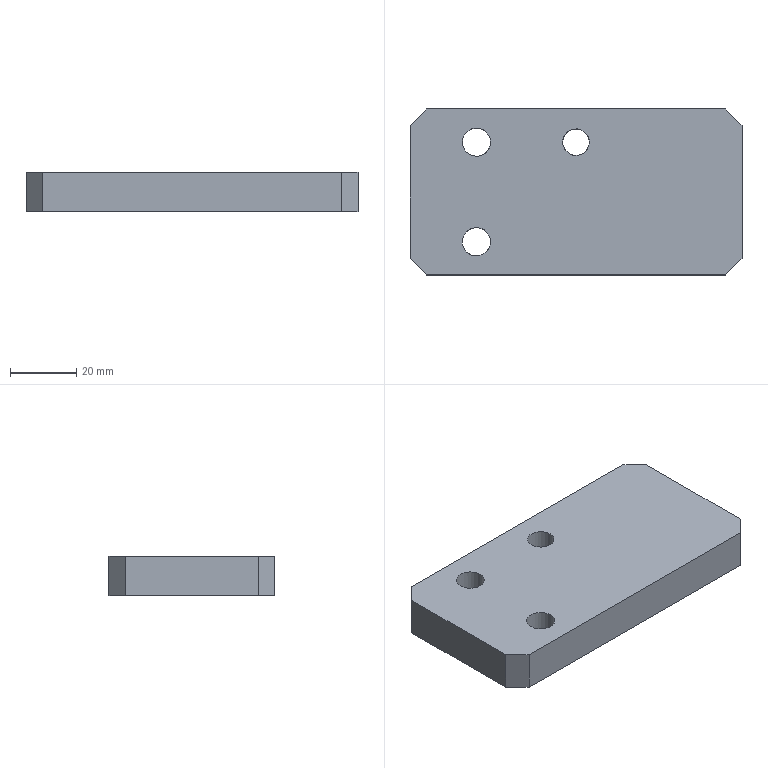Part | NX | features BREP 1 | 1 solid | 13 faces | box 100 x 50 x 12 mm | volume 57435 mm3 | plane 10 | cylinder 3 | commonest cylinder face diameters 8.5 x2 8 x1
STEP:
#1=CARTESIAN_POINT('',(50.,-20.,12.));
#2=VERTEX_POINT('',#1);
#3=CARTESIAN_POINT('',(50.,20.,12.));
#4=VERTEX_POINT('',#3);
#5=CARTESIAN_POINT('',(50.,25.,12.));
#6=DIRECTION('',(0.,1.,0.));
#7=VECTOR('',#6,1000.);
#8=LINE('',#5,#7);
#9=EDGE_CURVE('',#2,#4,#8,.T.);
#10=ORIENTED_EDGE('',*,*,#9,.F.);
#11=CARTESIAN_POINT('',(50.,-20.,0.));
#12=VERTEX_POINT('',#11);
#13=CARTESIAN_POINT('',(50.,-20.,15.));
#14=DIRECTION('',(0.,0.,-1.));
#15=VECTOR('',#14,1000.);
#16=LINE('',#13,#15);
#17=EDGE_CURVE('',#2,#12,#16,.T.);
#18=ORIENTED_EDGE('',*,*,#17,.T.);
#19=CARTESIAN_POINT('',(50.,20.,0.));
#20=VERTEX_POINT('',#19);
#21=CARTESIAN_POINT('',(50.,25.,0.));
#22=DIRECTION('',(0.,1.,0.));
#23=VECTOR('',#22,1000.);
#24=LINE('',#21,#23);
#25=EDGE_CURVE('',#12,#20,#24,.T.);
#26=ORIENTED_EDGE('',*,*,#25,.T.);
#27=CARTESIAN_POINT('',(50.,20.,15.));
#28=DIRECTION('',(0.,0.,1.));
#29=VECTOR('',#28,1000.);
#30=LINE('',#27,#29);
#31=EDGE_CURVE('',#20,#4,#30,.T.);
#32=ORIENTED_EDGE('',*,*,#31,.T.);
#33=EDGE_LOOP('',(#10,#18,#26,#32));
#34=FACE_BOUND('',#33,.T.);
#35=CARTESIAN_POINT('',(50.,25.,15.));
#36=DIRECTION('',(-1.,0.,0.));
#37=DIRECTION('',(0.,0.,-1.));
#38=AXIS2_PLACEMENT_3D('',#35,#36,#37);
#39=PLANE('',#38);
#40=ADVANCED_FACE('',(#34),#39,.F.);
#41=CARTESIAN_POINT('',(45.,25.,12.));
#42=VERTEX_POINT('',#41);
#43=CARTESIAN_POINT('',(-45.,25.,12.));
#44=VERTEX_POINT('',#43);
#45=CARTESIAN_POINT('',(-50.,25.,12.));
#46=DIRECTION('',(-1.,0.,0.));
#47=VECTOR('',#46,1000.);
#48=LINE('',#45,#47);
#49=EDGE_CURVE('',#42,#44,#48,.T.);
#50=ORIENTED_EDGE('',*,*,#49,.F.);
#51=CARTESIAN_POINT('',(45.,25.,0.));
#52=VERTEX_POINT('',#51);
#53=CARTESIAN_POINT('',(45.,25.,15.));
#54=DIRECTION('',(0.,0.,-1.));
#55=VECTOR('',#54,1000.);
#56=LINE('',#53,#55);
#57=EDGE_CURVE('',#42,#52,#56,.T.);
#58=ORIENTED_EDGE('',*,*,#57,.T.);
#59=CARTESIAN_POINT('',(-45.,25.,0.));
#60=VERTEX_POINT('',#59);
#61=CARTESIAN_POINT('',(-50.,25.,0.));
#62=DIRECTION('',(-1.,0.,0.));
#63=VECTOR('',#62,1000.);
#64=LINE('',#61,#63);
#65=EDGE_CURVE('',#52,#60,#64,.T.);
#66=ORIENTED_EDGE('',*,*,#65,.T.);
#67=CARTESIAN_POINT('',(-45.,25.,15.));
#68=DIRECTION('',(0.,0.,1.));
#69=VECTOR('',#68,1000.);
#70=LINE('',#67,#69);
#71=EDGE_CURVE('',#60,#44,#70,.T.);
#72=ORIENTED_EDGE('',*,*,#71,.T.);
#73=EDGE_LOOP('',(#50,#58,#66,#72));
#74=FACE_BOUND('',#73,.T.);
#75=CARTESIAN_POINT('',(-50.,25.,15.));
#76=DIRECTION('',(0.,-1.,0.));
#77=DIRECTION('',(0.,0.,1.));
#78=AXIS2_PLACEMENT_3D('',#75,#76,#77);
#79=PLANE('',#78);
#80=ADVANCED_FACE('',(#74),#79,.F.);
#81=CARTESIAN_POINT('',(-50.,20.,12.));
#82=VERTEX_POINT('',#81);
#83=CARTESIAN_POINT('',(-50.,-20.,12.));
#84=VERTEX_POINT('',#83);
#85=CARTESIAN_POINT('',(-50.,25.,12.));
#86=DIRECTION('',(0.,-1.,0.));
#87=VECTOR('',#86,1000.);
#88=LINE('',#85,#87);
#89=EDGE_CURVE('',#82,#84,#88,.T.);
#90=ORIENTED_EDGE('',*,*,#89,.F.);
#91=CARTESIAN_POINT('',(-50.,20.,0.));
#92=VERTEX_POINT('',#91);
#93=CARTESIAN_POINT('',(-50.,20.,15.));
#94=DIRECTION('',(0.,0.,-1.));
#95=VECTOR('',#94,1000.);
#96=LINE('',#93,#95);
#97=EDGE_CURVE('',#82,#92,#96,.T.);
#98=ORIENTED_EDGE('',*,*,#97,.T.);
#99=CARTESIAN_POINT('',(-50.,-20.,0.));
#100=VERTEX_POINT('',#99);
#101=CARTESIAN_POINT('',(-50.,25.,0.));
#102=DIRECTION('',(0.,-1.,0.));
#103=VECTOR('',#102,1000.);
#104=LINE('',#101,#103);
#105=EDGE_CURVE('',#92,#100,#104,.T.);
#106=ORIENTED_EDGE('',*,*,#105,.T.);
#107=CARTESIAN_POINT('',(-50.,-20.,15.));
#108=DIRECTION('',(0.,0.,1.));
#109=VECTOR('',#108,1000.);
#110=LINE('',#107,#109);
#111=EDGE_CURVE('',#100,#84,#110,.T.);
#112=ORIENTED_EDGE('',*,*,#111,.T.);
#113=EDGE_LOOP('',(#90,#98,#106,#112));
#114=FACE_BOUND('',#113,.T.);
#115=CARTESIAN_POINT('',(-50.,25.,15.));
#116=DIRECTION('',(1.,0.,0.));
#117=DIRECTION('',(0.,0.,1.));
#118=AXIS2_PLACEMENT_3D('',#115,#116,#117);
#119=PLANE('',#118);
#120=ADVANCED_FACE('',(#114),#119,.F.);
#121=CARTESIAN_POINT('',(-45.,-25.,12.));
#122=VERTEX_POINT('',#121);
#123=CARTESIAN_POINT('',(45.,-25.,12.));
#124=VERTEX_POINT('',#123);
#125=CARTESIAN_POINT('',(-50.,-25.,12.));
#126=DIRECTION('',(1.,0.,0.));
#127=VECTOR('',#126,1000.);
#128=LINE('',#125,#127);
#129=EDGE_CURVE('',#122,#124,#128,.T.);
#130=ORIENTED_EDGE('',*,*,#129,.F.);
#131=CARTESIAN_POINT('',(-45.,-25.,0.));
#132=VERTEX_POINT('',#131);
#133=CARTESIAN_POINT('',(-45.,-25.,15.));
#134=DIRECTION('',(0.,0.,-1.));
#135=VECTOR('',#134,1000.);
#136=LINE('',#133,#135);
#137=EDGE_CURVE('',#122,#132,#136,.T.);
#138=ORIENTED_EDGE('',*,*,#137,.T.);
#139=CARTESIAN_POINT('',(45.,-25.,0.));
#140=VERTEX_POINT('',#139);
#141=CARTESIAN_POINT('',(-50.,-25.,0.));
#142=DIRECTION('',(1.,0.,0.));
#143=VECTOR('',#142,1000.);
#144=LINE('',#141,#143);
#145=EDGE_CURVE('',#132,#140,#144,.T.);
#146=ORIENTED_EDGE('',*,*,#145,.T.);
#147=CARTESIAN_POINT('',(45.,-25.,15.));
#148=DIRECTION('',(0.,0.,1.));
#149=VECTOR('',#148,1000.);
#150=LINE('',#147,#149);
#151=EDGE_CURVE('',#140,#124,#150,.T.);
#152=ORIENTED_EDGE('',*,*,#151,.T.);
#153=EDGE_LOOP('',(#130,#138,#146,#152));
#154=FACE_BOUND('',#153,.T.);
#155=CARTESIAN_POINT('',(-50.,-25.,15.));
#156=DIRECTION('',(0.,1.,0.));
#157=DIRECTION('',(0.,0.,-1.));
#158=AXIS2_PLACEMENT_3D('',#155,#156,#157);
#159=PLANE('',#158);
#160=ADVANCED_FACE('',(#154),#159,.F.);
#161=ORIENTED_EDGE('',*,*,#137,.F.);
#162=CARTESIAN_POINT('',(-45.,-25.,12.));
#163=DIRECTION('',(-0.7071,0.7071,0.));
#164=VECTOR('',#163,1000.);
#165=LINE('',#162,#164);
#166=EDGE_CURVE('',#122,#84,#165,.T.);
#167=ORIENTED_EDGE('',*,*,#166,.T.);
#168=ORIENTED_EDGE('',*,*,#111,.F.);
#169=CARTESIAN_POINT('',(-45.,-25.,0.));
#170=DIRECTION('',(-0.7071,0.7071,0.));
#171=VECTOR('',#170,1000.);
#172=LINE('',#169,#171);
#173=EDGE_CURVE('',#132,#100,#172,.T.);
#174=ORIENTED_EDGE('',*,*,#173,.F.);
#175=EDGE_LOOP('',(#161,#167,#168,#174));
#176=FACE_BOUND('',#175,.T.);
#177=CARTESIAN_POINT('',(-45.,-25.,15.));
#178=DIRECTION('',(0.7071,0.7071,0.));
#179=DIRECTION('',(0.,0.,1.));
#180=AXIS2_PLACEMENT_3D('',#177,#178,#179);
#181=PLANE('',#180);
#182=ADVANCED_FACE('',(#176),#181,.F.);
#183=ORIENTED_EDGE('',*,*,#97,.F.);
#184=CARTESIAN_POINT('',(-50.,20.,12.));
#185=DIRECTION('',(0.7071,0.7071,0.));
#186=VECTOR('',#185,1000.);
#187=LINE('',#184,#186);
#188=EDGE_CURVE('',#82,#44,#187,.T.);
#189=ORIENTED_EDGE('',*,*,#188,.T.);
#190=ORIENTED_EDGE('',*,*,#71,.F.);
#191=CARTESIAN_POINT('',(-50.,20.,0.));
#192=DIRECTION('',(0.7071,0.7071,0.));
#193=VECTOR('',#192,1000.);
#194=LINE('',#191,#193);
#195=EDGE_CURVE('',#92,#60,#194,.T.);
#196=ORIENTED_EDGE('',*,*,#195,.F.);
#197=EDGE_LOOP('',(#183,#189,#190,#196));
#198=FACE_BOUND('',#197,.T.);
#199=CARTESIAN_POINT('',(-50.,20.,15.));
#200=DIRECTION('',(0.7071,-0.7071,0.));
#201=DIRECTION('',(0.,0.,1.));
#202=AXIS2_PLACEMENT_3D('',#199,#200,#201);
#203=PLANE('',#202);
#204=ADVANCED_FACE('',(#198),#203,.F.);
#205=ORIENTED_EDGE('',*,*,#17,.F.);
#206=CARTESIAN_POINT('',(50.,-20.,12.));
#207=DIRECTION('',(-0.7071,-0.7071,0.));
#208=VECTOR('',#207,1000.);
#209=LINE('',#206,#208);
#210=EDGE_CURVE('',#2,#124,#209,.T.);
#211=ORIENTED_EDGE('',*,*,#210,.T.);
#212=ORIENTED_EDGE('',*,*,#151,.F.);
#213=CARTESIAN_POINT('',(50.,-20.,0.));
#214=DIRECTION('',(-0.7071,-0.7071,0.));
#215=VECTOR('',#214,1000.);
#216=LINE('',#213,#215);
#217=EDGE_CURVE('',#12,#140,#216,.T.);
#218=ORIENTED_EDGE('',*,*,#217,.F.);
#219=EDGE_LOOP('',(#205,#211,#212,#218));
#220=FACE_BOUND('',#219,.T.);
#221=CARTESIAN_POINT('',(50.,-20.,15.));
#222=DIRECTION('',(-0.7071,0.7071,0.));
#223=DIRECTION('',(0.,0.,1.));
#224=AXIS2_PLACEMENT_3D('',#221,#222,#223);
#225=PLANE('',#224);
#226=ADVANCED_FACE('',(#220),#225,.F.);
#227=ORIENTED_EDGE('',*,*,#57,.F.);
#228=CARTESIAN_POINT('',(45.,25.,12.));
#229=DIRECTION('',(0.7071,-0.7071,0.));
#230=VECTOR('',#229,1000.);
#231=LINE('',#228,#230);
#232=EDGE_CURVE('',#42,#4,#231,.T.);
#233=ORIENTED_EDGE('',*,*,#232,.T.);
#234=ORIENTED_EDGE('',*,*,#31,.F.);
#235=CARTESIAN_POINT('',(45.,25.,0.));
#236=DIRECTION('',(0.7071,-0.7071,0.));
#237=VECTOR('',#236,1000.);
#238=LINE('',#235,#237);
#239=EDGE_CURVE('',#52,#20,#238,.T.);
#240=ORIENTED_EDGE('',*,*,#239,.F.);
#241=EDGE_LOOP('',(#227,#233,#234,#240));
#242=FACE_BOUND('',#241,.T.);
#243=CARTESIAN_POINT('',(45.,25.,15.));
#244=DIRECTION('',(-0.7071,-0.7071,0.));
#245=DIRECTION('',(0.,0.,1.));
#246=AXIS2_PLACEMENT_3D('',#243,#244,#245);
#247=PLANE('',#246);
#248=ADVANCED_FACE('',(#242),#247,.F.);
#249=CARTESIAN_POINT('',(-25.75,-15.,0.));
#250=VERTEX_POINT('',#249);
#251=CARTESIAN_POINT('',(-30.,-15.,0.));
#252=DIRECTION('',(0.,0.,1.));
#253=DIRECTION('',(1.,0.,0.));
#254=AXIS2_PLACEMENT_3D('',#251,#252,#253);
#255=CIRCLE('',#254,4.25);
#256=EDGE_CURVE('',#250,#250,#255,.T.);
#257=ORIENTED_EDGE('',*,*,#256,.T.);
#258=EDGE_LOOP('',(#257));
#259=FACE_BOUND('',#258,.T.);
#260=CARTESIAN_POINT('',(-25.75,15.,0.));
#261=VERTEX_POINT('',#260);
#262=CARTESIAN_POINT('',(-30.,15.,0.));
#263=DIRECTION('',(0.,0.,1.));
#264=DIRECTION('',(1.,0.,0.));
#265=AXIS2_PLACEMENT_3D('',#262,#263,#264);
#266=CIRCLE('',#265,4.25);
#267=EDGE_CURVE('',#261,#261,#266,.T.);
#268=ORIENTED_EDGE('',*,*,#267,.T.);
#269=EDGE_LOOP('',(#268));
#270=FACE_BOUND('',#269,.T.);
#271=CARTESIAN_POINT('',(4.,15.,0.));
#272=VERTEX_POINT('',#271);
#273=CARTESIAN_POINT('',(0.,15.,0.));
#274=DIRECTION('',(0.,0.,1.));
#275=DIRECTION('',(1.,0.,0.));
#276=AXIS2_PLACEMENT_3D('',#273,#274,#275);
#277=CIRCLE('',#276,4.);
#278=EDGE_CURVE('',#272,#272,#277,.T.);
#279=ORIENTED_EDGE('',*,*,#278,.T.);
#280=EDGE_LOOP('',(#279));
#281=FACE_BOUND('',#280,.T.);
#282=ORIENTED_EDGE('',*,*,#145,.F.);
#283=ORIENTED_EDGE('',*,*,#173,.T.);
#284=ORIENTED_EDGE('',*,*,#105,.F.);
#285=ORIENTED_EDGE('',*,*,#195,.T.);
#286=ORIENTED_EDGE('',*,*,#65,.F.);
#287=ORIENTED_EDGE('',*,*,#239,.T.);
#288=ORIENTED_EDGE('',*,*,#25,.F.);
#289=ORIENTED_EDGE('',*,*,#217,.T.);
#290=EDGE_LOOP('',(#282,#283,#284,#285,#286,#287,#288,#289));
#291=FACE_BOUND('',#290,.T.);
#292=CARTESIAN_POINT('',(0.,0.,0.));
#293=DIRECTION('',(0.,0.,1.));
#294=DIRECTION('',(-1.,0.,0.));
#295=AXIS2_PLACEMENT_3D('',#292,#293,#294);
#296=PLANE('',#295);
#297=ADVANCED_FACE('',(#259,#270,#281,#291),#296,.F.);
#298=CARTESIAN_POINT('',(-30.,-19.25,12.));
#299=VERTEX_POINT('',#298);
#300=CARTESIAN_POINT('',(-30.,-15.,12.));
#301=DIRECTION('',(0.,0.,1.));
#302=DIRECTION('',(0.,-1.,0.));
#303=AXIS2_PLACEMENT_3D('',#300,#301,#302);
#304=CIRCLE('',#303,4.25);
#305=EDGE_CURVE('',#299,#299,#304,.T.);
#306=ORIENTED_EDGE('',*,*,#305,.F.);
#307=EDGE_LOOP('',(#306));
#308=FACE_BOUND('',#307,.T.);
#309=CARTESIAN_POINT('',(-30.,10.75,12.));
#310=VERTEX_POINT('',#309);
#311=CARTESIAN_POINT('',(-30.,15.,12.));
#312=DIRECTION('',(0.,0.,1.));
#313=DIRECTION('',(0.,-1.,0.));
#314=AXIS2_PLACEMENT_3D('',#311,#312,#313);
#315=CIRCLE('',#314,4.25);
#316=EDGE_CURVE('',#310,#310,#315,.T.);
#317=ORIENTED_EDGE('',*,*,#316,.F.);
#318=EDGE_LOOP('',(#317));
#319=FACE_BOUND('',#318,.T.);
#320=CARTESIAN_POINT('',(0.,11.,12.));
#321=VERTEX_POINT('',#320);
#322=CARTESIAN_POINT('',(0.,15.,12.));
#323=DIRECTION('',(0.,0.,1.));
#324=DIRECTION('',(0.,-1.,0.));
#325=AXIS2_PLACEMENT_3D('',#322,#323,#324);
#326=CIRCLE('',#325,4.);
#327=EDGE_CURVE('',#321,#321,#326,.T.);
#328=ORIENTED_EDGE('',*,*,#327,.F.);
#329=EDGE_LOOP('',(#328));
#330=FACE_BOUND('',#329,.T.);
#331=ORIENTED_EDGE('',*,*,#129,.T.);
#332=ORIENTED_EDGE('',*,*,#210,.F.);
#333=ORIENTED_EDGE('',*,*,#9,.T.);
#334=ORIENTED_EDGE('',*,*,#232,.F.);
#335=ORIENTED_EDGE('',*,*,#49,.T.);
#336=ORIENTED_EDGE('',*,*,#188,.F.);
#337=ORIENTED_EDGE('',*,*,#89,.T.);
#338=ORIENTED_EDGE('',*,*,#166,.F.);
#339=EDGE_LOOP('',(#331,#332,#333,#334,#335,#336,#337,#338));
#340=FACE_BOUND('',#339,.T.);
#341=CARTESIAN_POINT('',(250.,380.,12.));
#342=DIRECTION('',(0.,0.,1.));
#343=DIRECTION('',(0.,1.,0.));
#344=AXIS2_PLACEMENT_3D('',#341,#342,#343);
#345=PLANE('',#344);
#346=ADVANCED_FACE('',(#308,#319,#330,#340),#345,.T.);
#347=ORIENTED_EDGE('',*,*,#327,.T.);
#348=EDGE_LOOP('',(#347));
#349=FACE_BOUND('',#348,.T.);
#350=ORIENTED_EDGE('',*,*,#278,.F.);
#351=EDGE_LOOP('',(#350));
#352=FACE_BOUND('',#351,.T.);
#353=CARTESIAN_POINT('',(0.,15.,12.));
#354=DIRECTION('',(0.,0.,1.));
#355=DIRECTION('',(0.,1.,0.));
#356=AXIS2_PLACEMENT_3D('',#353,#354,#355);
#357=CYLINDRICAL_SURFACE('',#356,4.);
#358=ADVANCED_FACE('',(#349,#352),#357,.F.);
#359=ORIENTED_EDGE('',*,*,#316,.T.);
#360=EDGE_LOOP('',(#359));
#361=FACE_BOUND('',#360,.T.);
#362=ORIENTED_EDGE('',*,*,#267,.F.);
#363=EDGE_LOOP('',(#362));
#364=FACE_BOUND('',#363,.T.);
#365=CARTESIAN_POINT('',(-30.,15.,12.));
#366=DIRECTION('',(0.,0.,1.));
#367=DIRECTION('',(0.,1.,0.));
#368=AXIS2_PLACEMENT_3D('',#365,#366,#367);
#369=CYLINDRICAL_SURFACE('',#368,4.25);
#370=ADVANCED_FACE('',(#361,#364),#369,.F.);
#371=ORIENTED_EDGE('',*,*,#305,.T.);
#372=EDGE_LOOP('',(#371));
#373=FACE_BOUND('',#372,.T.);
#374=ORIENTED_EDGE('',*,*,#256,.F.);
#375=EDGE_LOOP('',(#374));
#376=FACE_BOUND('',#375,.T.);
#377=CARTESIAN_POINT('',(-30.,-15.,12.));
#378=DIRECTION('',(0.,0.,1.));
#379=DIRECTION('',(0.,1.,0.));
#380=AXIS2_PLACEMENT_3D('',#377,#378,#379);
#381=CYLINDRICAL_SURFACE('',#380,4.25);
#382=ADVANCED_FACE('',(#373,#376),#381,.F.);
#383=CLOSED_SHELL('',(#40,#80,#120,#160,#182,#204,#226,#248,#297,#346,#358,#370,#382));
#384=MANIFOLD_SOLID_BREP('',#383);
#385=(LENGTH_UNIT()NAMED_UNIT(*)SI_UNIT(.MILLI.,.METRE.));
#386=UNCERTAINTY_MEASURE_WITH_UNIT(LENGTH_MEASURE(0.00001),#385,'','');
#387=(NAMED_UNIT(*)PLANE_ANGLE_UNIT()SI_UNIT($,.RADIAN.));
#388=(NAMED_UNIT(*)SI_UNIT($,.STERADIAN.)SOLID_ANGLE_UNIT());
#389=(GEOMETRIC_REPRESENTATION_CONTEXT(3)GLOBAL_UNCERTAINTY_ASSIGNED_CONTEXT((#386))GLOBAL_UNIT_ASSIGNED_CONTEXT((#385,#387,#388))REPRESENTATION_CONTEXT('',''));
#390=ADVANCED_BREP_SHAPE_REPRESENTATION('',(#384),#389);